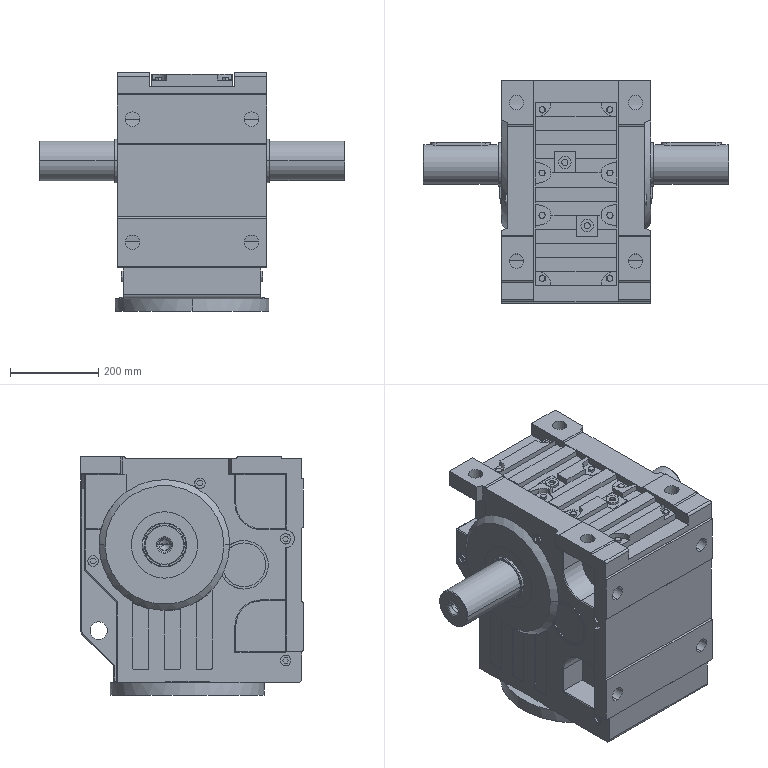Part | STEP file | 3 solids | 660 faces | box 694 x 505 x 541 mm | volume 76306472 mm3 | plane 348 | cylinder 200 | cone 84 | torus 22 | sphere 6 | commonest cylinder face diameters 4 x58 24 x20 33 x16 29.25 x12 6 x10 25 x8